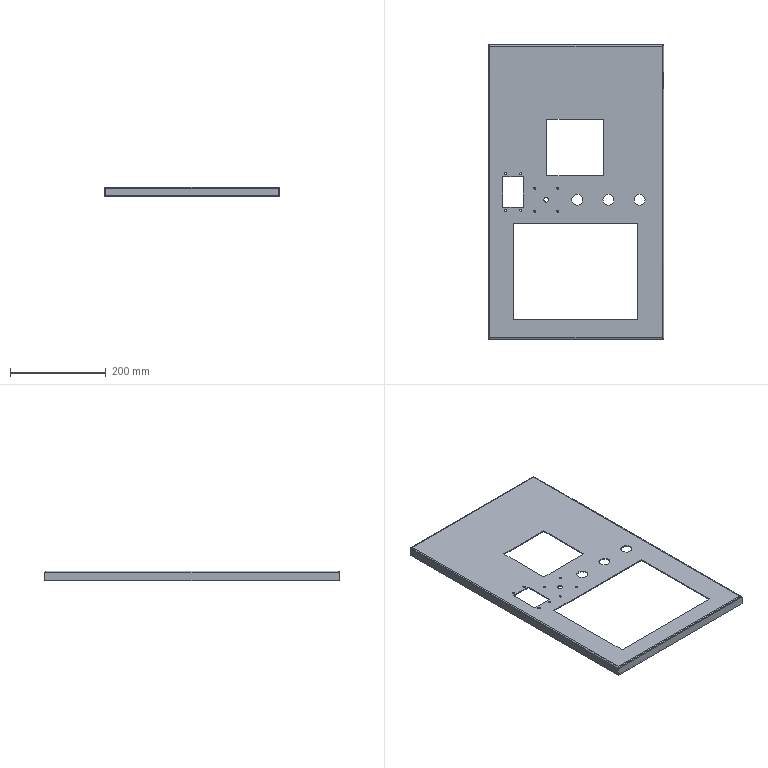Part | SolidWorks | features ICE 6, HoleWzd 3, Cut 1, Extrusion 1, Fillet 1, MirrorPattern 1, Shell 1 | 1 solid | 68 faces | box 365.5 x 614 x 20 mm | volume 436625 mm3 | plane 40 | cylinder 28 | commonest cylinder face diameters 4.2 x8 4.5 x8 23 x6 6 x4 10 x2